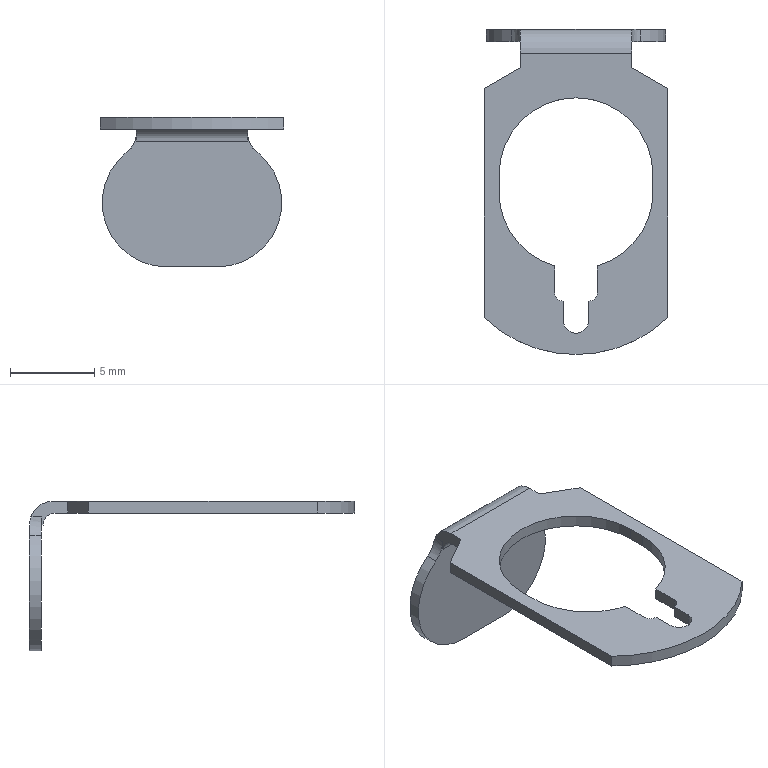Part | SolidWorks | features BaseBody 1 | 1 solid | 86 faces | box 10.922 x 19.304 x 8.89 mm | volume 127.415 mm3 | plane 67 | cylinder 19 | commonest cylinder face diameters 2.845 x3 9.144 x3 1.016 x2 7.62 x2 0.157 x1 0.385 x1